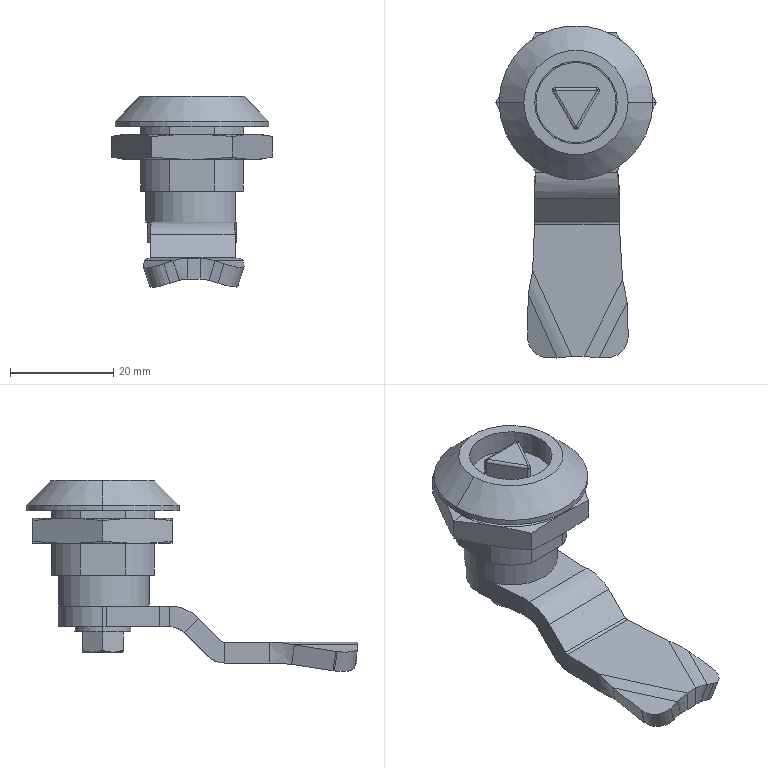Part | SolidWorks | features BaseBody 5 | 5 solids | 137 faces | box 31.177 x 64.298 x 36.976 mm | volume 13076 mm3 | plane 68 | cylinder 42 | sphere 13 | cone 8 | spline 6 | commonest cylinder face diameters 1 x7 8 x6 16 x5 21.7 x4 6.34 x3 17.25 x3